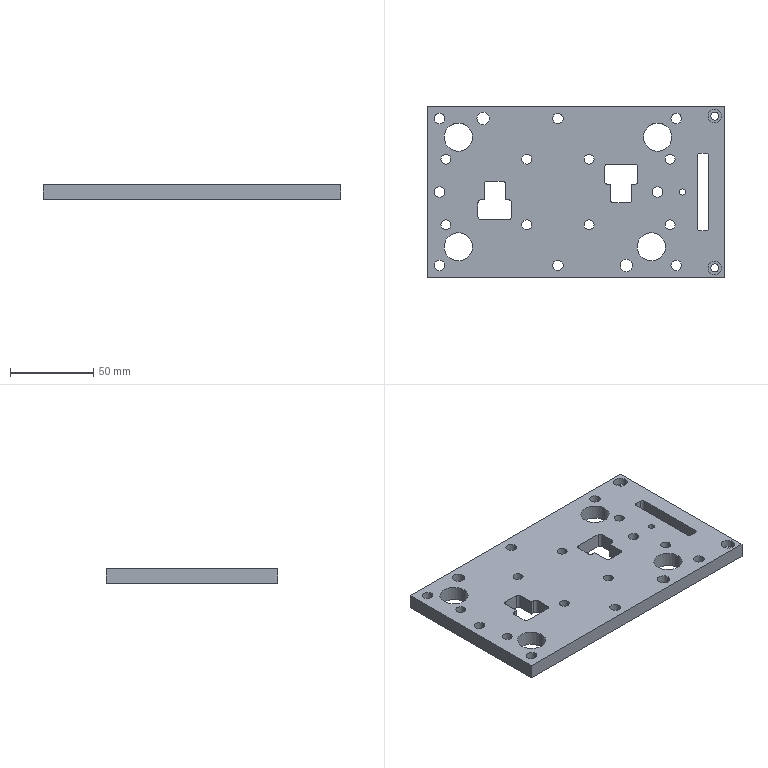Part | Creo | features DATUM PLANE 3, CURVE 2, COORDINATE SYSTEM 1, CUT 1, PROTRUSION 1 | 1 solid | 98 faces | box 179.25 x 103.5 x 9 mm | volume 143240 mm3 | cylinder 70 | plane 28 | commonest cylinder face diameters 6 x16 6.375 x16 3.75 x14 17 x8 3 x4 4.875 x4